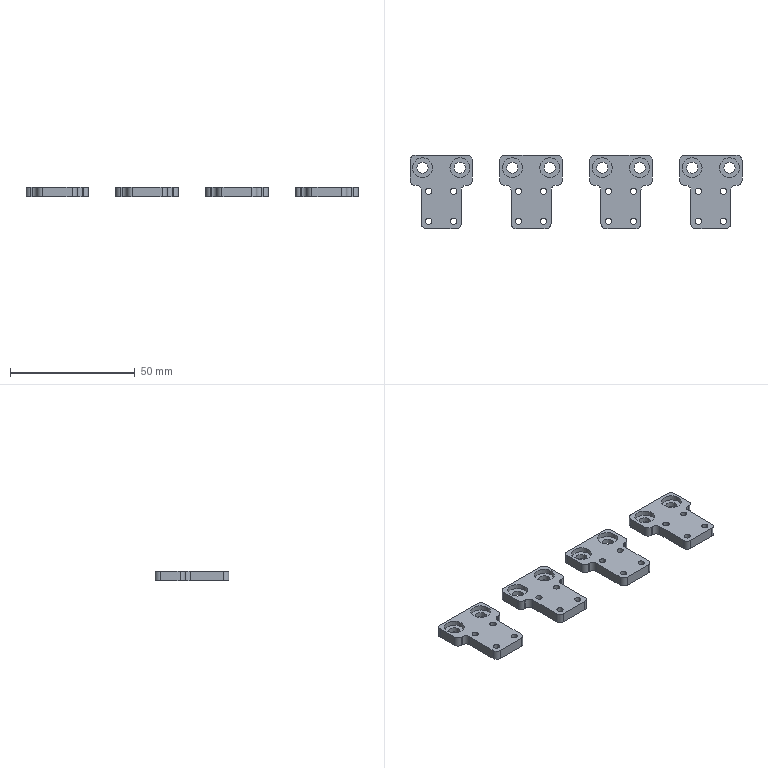CAM job | NX | 3-axis milling, drilling | part box 133 x 29.5 x 4 mm | stock box 138 x 30.5 x 8 mm
Tools:
number,name,description,diameter,corner_radius,flute_length,length,flutes
4,D4,平底铣刀-粗,4.0,0.0,25.0,75.0,2
9,D10,平底铣刀-粗,10.0,0.0,35.0,75.0,2
11,D4-J,平底铣刀-精,4.0,0.0,50.0,75.0,2
7,D6-J,平底铣刀-精,6.0,0.0,25.0,75.0,2
1,D80R0.8飞刀,圆鼻刀-粗,80.0,0.8,50.0,75.0,2
1,D80R0.8飞刀-J,圆鼻刀-精,80.0,0.8,50.0,75.0,2
2,D6倒角刀,倒角刀,6.0,0.0,3.0,25.0,2
20,M3X0.5,丝锥,2.5,0.0,35.0,50.0,2
12,ZT2.5,钻头,2.5,0.0,35.0,50.0,2
11,ZT4.5,钻头,4.5,0.0,35.0,50.0,2
Operations:
program,operation,operation_type,tool,method,geometry_group,spindle_rpm,surface_speed,feed_per_tooth,feed_cut,feed_plunge,cut_length_mm,path_length_mm,cut_time_min,machine_time_min
B,底壁铣飞面一刀开粗_COPY,VolumeBased25DMillingOperation,D80R0.8飞刀,分层开粗-切深K-步距G,W-B,2800.0,703.696,0.5357,3000.0,100.0,1685.433,3242.005,0.5618,0.7175
B,底壁铣飞面一刀精光_COPY,VolumeBased25DMillingOperation,D80R0.8飞刀-J,侧刃精光-切深K-步距G,W-B,4000.0,1005.28,0.125,1000.0,100.0,240.579,276.579,0.2406,0.2442
B,钻倒角_2,Operation,D6倒角刀,METHOD,W-B,8000.0,150.796,0.0625,1000.0,0.0,76.0,452.375,0.076,0.1136
B,钻倒角_3,Operation,D6倒角刀,METHOD,W-B,8000.0,150.796,0.0625,1000.0,0.0,44.4,274.628,0.0444,0.0674
B,C0.3封闭铣廓倒角6X45L_COPY,PlanarMilling,D6倒角刀,爬面_倒角-切深0-步距G,W-B,7000.0,131.0,0.1071,1500.0,100.0,480.314,735.214,0.3202,0.3457
A,顶面,FaceMilling,D80R0.8飞刀,侧刃精光-切深K-步距G,W-A,4000.0,1005.31,0.125,1000.0,100.0,227.0,263.0,0.227,0.2306
A,外形粗_2,VolumeBased25DMillingOperation,D10,METHOD,W-A,8000.0,251.327,0.3125,5000.0,80.0,5830.686,6111.386,1.166,1.194
A,打点-深0.8,Operation,D6倒角刀,NONE,W-A,8000.0,150.796,0.0312,500.0,90.0,43.2,427.997,0.0864,0.1249
A,通孔-M3螺纹底孔,Operation,ZT2.5,NONE,W-A,3000.0,23.562,0.05,300.0,90.0,172.017,609.641,0.5734,0.6172
A,沉头孔-钻孔0段,Operation,ZT4.5,NONE,W-A,2800.0,39.584,0.0179,100.0,90.0,66.816,303.836,0.6682,0.6919
A,铣孔开粗D4_1,CylinderMilling,D4,NONE,W-A,8000.0,100.531,0.075,1200.0,100.0,939.378,1430.378,0.7828,0.8319
A,铣孔精光D4_1,CylinderMilling,D4-J,精光步距切深关,W-A,8000.0,100.531,0.0312,500.0,100.0,204.435,695.434,0.4089,0.458
A,外形侧面,ZLevelMilling,D4-J,METHOD,W-A,9000.0,84.823,0.1389,2500.0,80.0,1006.769,1601.505,0.4036,0.4631
A,仅选体,SurfaceContour,D6倒角刀,METHOD,W-A,8000.0,150.796,0.1875,3000.0,100.0,477.79,727.497,0.1593,0.1842
A,钻倒角_1,Operation,D6倒角刀,METHOD,W-A,8000.0,150.796,0.0312,500.0,0.0,76.0,452.375,0.152,0.1896
A,铣倒角_1,PlanarMilling,D6倒角刀,NONE,W-A,8000.0,150.796,0.0312,500.0,100.0,271.743,637.948,0.5435,0.5801
A,通孔-攻牙M3,Operation,M3X0.5,METHOD,W-A,800.0,6.283,0.0003,0.5,90.0,128.0,521.606,256.0,256.039
A,外形半精_2,VolumeBased25DMillingOperation,D6-J,METHOD,W-A,8000.0,251.327,0.0625,1000.0,100.0,500.522,806.462,0.5005,0.5311
A,底壁铣精光侧面-中_COPY,VolumeBased25DMillingOperation,D6-J,侧刃精光-切深K-步距G,W-A,8000.0,150.792,0.0625,1000.0,100.0,147.002,403.974,0.147,0.1727